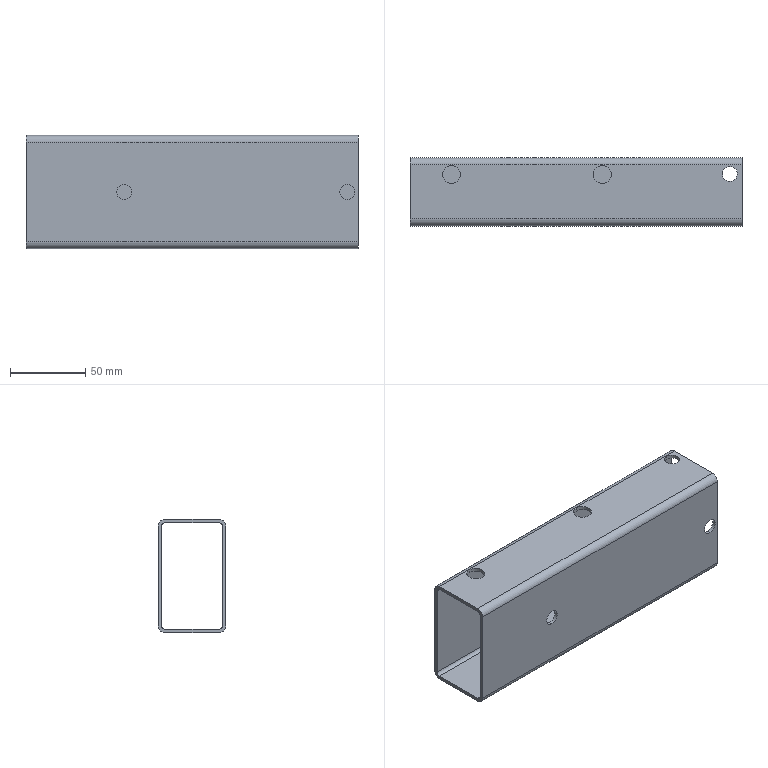Part | STEP file | [06] | 1 solid | 30 faces | box 220 x 45 x 75 mm | volume 112545 mm3 | cylinder 20 | plane 10 | commonest cylinder face diameters 10 x8 4.6 x4 9.2 x4 12 x4
STEP:
#1=CARTESIAN_POINT('',(65.,0.,42.5));
#2=VERTEX_POINT('',#1);
#3=CARTESIAN_POINT('',(65.,0.,32.5));
#4=VERTEX_POINT('',#3);
#5=CARTESIAN_POINT('',(65.,0.,37.5));
#6=DIRECTION('',(0.,1.,0.));
#7=DIRECTION('',(0.,0.,-1.));
#8=AXIS2_PLACEMENT_3D('',#5,#6,#7);
#9=CIRCLE('',#8,5.);
#10=EDGE_CURVE('',#2,#4,#9,.T.);
#11=ORIENTED_EDGE('',*,*,#10,.F.);
#12=CARTESIAN_POINT('',(65.,2.3,42.5));
#13=VERTEX_POINT('',#12);
#14=CARTESIAN_POINT('',(65.,0.,42.5));
#15=DIRECTION('',(0.,1.,0.));
#16=VECTOR('',#15,1000.);
#17=LINE('',#14,#16);
#18=EDGE_CURVE('',#2,#13,#17,.T.);
#19=ORIENTED_EDGE('',*,*,#18,.T.);
#20=CARTESIAN_POINT('',(65.,2.3,32.5));
#21=VERTEX_POINT('',#20);
#22=CARTESIAN_POINT('',(65.,2.3,37.5));
#23=DIRECTION('',(0.,-1.,0.));
#24=DIRECTION('',(0.,0.,1.));
#25=AXIS2_PLACEMENT_3D('',#22,#23,#24);
#26=CIRCLE('',#25,5.);
#27=EDGE_CURVE('',#21,#13,#26,.T.);
#28=ORIENTED_EDGE('',*,*,#27,.F.);
#29=CARTESIAN_POINT('',(65.,0.,32.5));
#30=DIRECTION('',(0.,1.,0.));
#31=VECTOR('',#30,1000.);
#32=LINE('',#29,#31);
#33=EDGE_CURVE('',#4,#21,#32,.T.);
#34=ORIENTED_EDGE('',*,*,#33,.F.);
#35=EDGE_LOOP('',(#11,#19,#28,#34));
#36=FACE_OUTER_BOUND('',#35,.T.);
#37=CARTESIAN_POINT('',(65.,0.,37.5));
#38=DIRECTION('',(0.,1.,0.));
#39=DIRECTION('',(0.,0.,-1.));
#40=AXIS2_PLACEMENT_3D('',#37,#38,#39);
#41=CYLINDRICAL_SURFACE('',#40,5.);
#42=ADVANCED_FACE('',(#36),#41,.F.);
#43=CARTESIAN_POINT('',(213.,0.,42.5));
#44=VERTEX_POINT('',#43);
#45=CARTESIAN_POINT('',(213.,0.,32.5));
#46=VERTEX_POINT('',#45);
#47=CARTESIAN_POINT('',(213.,0.,37.5));
#48=DIRECTION('',(0.,1.,0.));
#49=DIRECTION('',(0.,0.,-1.));
#50=AXIS2_PLACEMENT_3D('',#47,#48,#49);
#51=CIRCLE('',#50,5.);
#52=EDGE_CURVE('',#44,#46,#51,.T.);
#53=ORIENTED_EDGE('',*,*,#52,.F.);
#54=CARTESIAN_POINT('',(213.,2.3,42.5));
#55=VERTEX_POINT('',#54);
#56=CARTESIAN_POINT('',(213.,0.,42.5));
#57=DIRECTION('',(0.,1.,0.));
#58=VECTOR('',#57,1000.);
#59=LINE('',#56,#58);
#60=EDGE_CURVE('',#44,#55,#59,.T.);
#61=ORIENTED_EDGE('',*,*,#60,.T.);
#62=CARTESIAN_POINT('',(213.,2.3,32.5));
#63=VERTEX_POINT('',#62);
#64=CARTESIAN_POINT('',(213.,2.3,37.5));
#65=DIRECTION('',(0.,-1.,0.));
#66=DIRECTION('',(0.,0.,1.));
#67=AXIS2_PLACEMENT_3D('',#64,#65,#66);
#68=CIRCLE('',#67,5.);
#69=EDGE_CURVE('',#63,#55,#68,.T.);
#70=ORIENTED_EDGE('',*,*,#69,.F.);
#71=CARTESIAN_POINT('',(213.,0.,32.5));
#72=DIRECTION('',(0.,1.,0.));
#73=VECTOR('',#72,1000.);
#74=LINE('',#71,#73);
#75=EDGE_CURVE('',#46,#63,#74,.T.);
#76=ORIENTED_EDGE('',*,*,#75,.F.);
#77=EDGE_LOOP('',(#53,#61,#70,#76));
#78=FACE_OUTER_BOUND('',#77,.T.);
#79=CARTESIAN_POINT('',(213.,0.,37.5));
#80=DIRECTION('',(0.,1.,0.));
#81=DIRECTION('',(0.,0.,-1.));
#82=AXIS2_PLACEMENT_3D('',#79,#80,#81);
#83=CYLINDRICAL_SURFACE('',#82,5.);
#84=ADVANCED_FACE('',(#78),#83,.F.);
#85=CARTESIAN_POINT('',(212.,39.5,2.3));
#86=VERTEX_POINT('',#85);
#87=CARTESIAN_POINT('',(212.,29.5,2.3));
#88=VERTEX_POINT('',#87);
#89=CARTESIAN_POINT('',(212.,34.5,2.3));
#90=DIRECTION('',(0.,0.,-1.));
#91=DIRECTION('',(0.,-1.,0.));
#92=AXIS2_PLACEMENT_3D('',#89,#90,#91);
#93=CIRCLE('',#92,5.);
#94=EDGE_CURVE('',#86,#88,#93,.T.);
#95=ORIENTED_EDGE('',*,*,#94,.F.);
#96=CARTESIAN_POINT('',(212.,39.5,0.));
#97=VERTEX_POINT('',#96);
#98=CARTESIAN_POINT('',(212.,39.5,2.3));
#99=DIRECTION('',(0.,0.,-1.));
#100=VECTOR('',#99,1000.);
#101=LINE('',#98,#100);
#102=EDGE_CURVE('',#86,#97,#101,.T.);
#103=ORIENTED_EDGE('',*,*,#102,.T.);
#104=CARTESIAN_POINT('',(212.,29.5,0.));
#105=VERTEX_POINT('',#104);
#106=CARTESIAN_POINT('',(212.,34.5,0.));
#107=DIRECTION('',(0.,0.,1.));
#108=DIRECTION('',(0.,1.,0.));
#109=AXIS2_PLACEMENT_3D('',#106,#107,#108);
#110=CIRCLE('',#109,5.);
#111=EDGE_CURVE('',#105,#97,#110,.T.);
#112=ORIENTED_EDGE('',*,*,#111,.F.);
#113=CARTESIAN_POINT('',(212.,29.5,2.3));
#114=DIRECTION('',(0.,0.,-1.));
#115=VECTOR('',#114,1000.);
#116=LINE('',#113,#115);
#117=EDGE_CURVE('',#88,#105,#116,.T.);
#118=ORIENTED_EDGE('',*,*,#117,.F.);
#119=EDGE_LOOP('',(#95,#103,#112,#118));
#120=FACE_OUTER_BOUND('',#119,.T.);
#121=CARTESIAN_POINT('',(212.,34.5,2.3));
#122=DIRECTION('',(0.,0.,-1.));
#123=DIRECTION('',(0.,-1.,0.));
#124=AXIS2_PLACEMENT_3D('',#121,#122,#123);
#125=CYLINDRICAL_SURFACE('',#124,5.);
#126=ADVANCED_FACE('',(#120),#125,.F.);
#127=CARTESIAN_POINT('',(212.,39.5,75.));
#128=VERTEX_POINT('',#127);
#129=CARTESIAN_POINT('',(212.,29.5,75.));
#130=VERTEX_POINT('',#129);
#131=CARTESIAN_POINT('',(212.,34.5,75.));
#132=DIRECTION('',(0.,0.,-1.));
#133=DIRECTION('',(0.,-1.,0.));
#134=AXIS2_PLACEMENT_3D('',#131,#132,#133);
#135=CIRCLE('',#134,5.);
#136=EDGE_CURVE('',#128,#130,#135,.T.);
#137=ORIENTED_EDGE('',*,*,#136,.F.);
#138=CARTESIAN_POINT('',(212.,39.5,72.7));
#139=VERTEX_POINT('',#138);
#140=CARTESIAN_POINT('',(212.,39.5,75.));
#141=DIRECTION('',(0.,0.,-1.));
#142=VECTOR('',#141,1000.);
#143=LINE('',#140,#142);
#144=EDGE_CURVE('',#128,#139,#143,.T.);
#145=ORIENTED_EDGE('',*,*,#144,.T.);
#146=CARTESIAN_POINT('',(212.,29.5,72.7));
#147=VERTEX_POINT('',#146);
#148=CARTESIAN_POINT('',(212.,34.5,72.7));
#149=DIRECTION('',(0.,0.,1.));
#150=DIRECTION('',(0.,1.,0.));
#151=AXIS2_PLACEMENT_3D('',#148,#149,#150);
#152=CIRCLE('',#151,5.);
#153=EDGE_CURVE('',#147,#139,#152,.T.);
#154=ORIENTED_EDGE('',*,*,#153,.F.);
#155=CARTESIAN_POINT('',(212.,29.5,75.));
#156=DIRECTION('',(0.,0.,-1.));
#157=VECTOR('',#156,1000.);
#158=LINE('',#155,#157);
#159=EDGE_CURVE('',#130,#147,#158,.T.);
#160=ORIENTED_EDGE('',*,*,#159,.F.);
#161=EDGE_LOOP('',(#137,#145,#154,#160));
#162=FACE_OUTER_BOUND('',#161,.T.);
#163=CARTESIAN_POINT('',(212.,34.5,75.));
#164=DIRECTION('',(0.,0.,-1.));
#165=DIRECTION('',(0.,-1.,0.));
#166=AXIS2_PLACEMENT_3D('',#163,#164,#165);
#167=CYLINDRICAL_SURFACE('',#166,5.);
#168=ADVANCED_FACE('',(#162),#167,.F.);
#169=CARTESIAN_POINT('',(127.5,40.,75.));
#170=VERTEX_POINT('',#169);
#171=CARTESIAN_POINT('',(127.5,28.,75.));
#172=VERTEX_POINT('',#171);
#173=CARTESIAN_POINT('',(127.5,34.,75.));
#174=DIRECTION('',(0.,0.,-1.));
#175=DIRECTION('',(0.,-1.,0.));
#176=AXIS2_PLACEMENT_3D('',#173,#174,#175);
#177=CIRCLE('',#176,6.);
#178=EDGE_CURVE('',#170,#172,#177,.T.);
#179=ORIENTED_EDGE('',*,*,#178,.F.);
#180=CARTESIAN_POINT('',(127.5,40.,72.7));
#181=VERTEX_POINT('',#180);
#182=CARTESIAN_POINT('',(127.5,40.,75.));
#183=DIRECTION('',(0.,0.,-1.));
#184=VECTOR('',#183,1000.);
#185=LINE('',#182,#184);
#186=EDGE_CURVE('',#170,#181,#185,.T.);
#187=ORIENTED_EDGE('',*,*,#186,.T.);
#188=CARTESIAN_POINT('',(127.5,28.,72.7));
#189=VERTEX_POINT('',#188);
#190=CARTESIAN_POINT('',(127.5,34.,72.7));
#191=DIRECTION('',(0.,0.,1.));
#192=DIRECTION('',(0.,1.,0.));
#193=AXIS2_PLACEMENT_3D('',#190,#191,#192);
#194=CIRCLE('',#193,6.);
#195=EDGE_CURVE('',#189,#181,#194,.T.);
#196=ORIENTED_EDGE('',*,*,#195,.F.);
#197=CARTESIAN_POINT('',(127.5,28.,75.));
#198=DIRECTION('',(0.,0.,-1.));
#199=VECTOR('',#198,1000.);
#200=LINE('',#197,#199);
#201=EDGE_CURVE('',#172,#189,#200,.T.);
#202=ORIENTED_EDGE('',*,*,#201,.F.);
#203=EDGE_LOOP('',(#179,#187,#196,#202));
#204=FACE_OUTER_BOUND('',#203,.T.);
#205=CARTESIAN_POINT('',(127.5,34.,75.));
#206=DIRECTION('',(0.,0.,-1.));
#207=DIRECTION('',(0.,-1.,0.));
#208=AXIS2_PLACEMENT_3D('',#205,#206,#207);
#209=CYLINDRICAL_SURFACE('',#208,6.);
#210=ADVANCED_FACE('',(#204),#209,.F.);
#211=CARTESIAN_POINT('',(27.5,40.,75.));
#212=VERTEX_POINT('',#211);
#213=CARTESIAN_POINT('',(27.5,28.,75.));
#214=VERTEX_POINT('',#213);
#215=CARTESIAN_POINT('',(27.5,34.,75.));
#216=DIRECTION('',(0.,0.,-1.));
#217=DIRECTION('',(0.,-1.,0.));
#218=AXIS2_PLACEMENT_3D('',#215,#216,#217);
#219=CIRCLE('',#218,6.);
#220=EDGE_CURVE('',#212,#214,#219,.T.);
#221=ORIENTED_EDGE('',*,*,#220,.F.);
#222=CARTESIAN_POINT('',(27.5,40.,72.7));
#223=VERTEX_POINT('',#222);
#224=CARTESIAN_POINT('',(27.5,40.,75.));
#225=DIRECTION('',(0.,0.,-1.));
#226=VECTOR('',#225,1000.);
#227=LINE('',#224,#226);
#228=EDGE_CURVE('',#212,#223,#227,.T.);
#229=ORIENTED_EDGE('',*,*,#228,.T.);
#230=CARTESIAN_POINT('',(27.5,28.,72.7));
#231=VERTEX_POINT('',#230);
#232=CARTESIAN_POINT('',(27.5,34.,72.7));
#233=DIRECTION('',(0.,0.,1.));
#234=DIRECTION('',(0.,1.,0.));
#235=AXIS2_PLACEMENT_3D('',#232,#233,#234);
#236=CIRCLE('',#235,6.);
#237=EDGE_CURVE('',#231,#223,#236,.T.);
#238=ORIENTED_EDGE('',*,*,#237,.F.);
#239=CARTESIAN_POINT('',(27.5,28.,75.));
#240=DIRECTION('',(0.,0.,-1.));
#241=VECTOR('',#240,1000.);
#242=LINE('',#239,#241);
#243=EDGE_CURVE('',#214,#231,#242,.T.);
#244=ORIENTED_EDGE('',*,*,#243,.F.);
#245=EDGE_LOOP('',(#221,#229,#238,#244));
#246=FACE_OUTER_BOUND('',#245,.T.);
#247=CARTESIAN_POINT('',(27.5,34.,75.));
#248=DIRECTION('',(0.,0.,-1.));
#249=DIRECTION('',(0.,-1.,0.));
#250=AXIS2_PLACEMENT_3D('',#247,#248,#249);
#251=CYLINDRICAL_SURFACE('',#250,6.);
#252=ADVANCED_FACE('',(#246),#251,.F.);
#253=CARTESIAN_POINT('',(0.,45.,70.4));
#254=VERTEX_POINT('',#253);
#255=CARTESIAN_POINT('',(0.,45.,4.6));
#256=VERTEX_POINT('',#255);
#257=CARTESIAN_POINT('',(0.,45.,70.4));
#258=DIRECTION('',(0.,0.,-1.));
#259=VECTOR('',#258,1000.);
#260=LINE('',#257,#259);
#261=EDGE_CURVE('',#254,#256,#260,.T.);
#262=ORIENTED_EDGE('',*,*,#261,.T.);
#263=CARTESIAN_POINT('',(0.,40.4,0.));
#264=VERTEX_POINT('',#263);
#265=CARTESIAN_POINT('',(0.,40.4,4.6));
#266=DIRECTION('',(-1.,0.,0.));
#267=DIRECTION('',(0.,1.,0.));
#268=AXIS2_PLACEMENT_3D('',#265,#266,#267);
#269=CIRCLE('',#268,4.6);
#270=EDGE_CURVE('',#256,#264,#269,.T.);
#271=ORIENTED_EDGE('',*,*,#270,.T.);
#272=CARTESIAN_POINT('',(0.,4.6,0.));
#273=VERTEX_POINT('',#272);
#274=CARTESIAN_POINT('',(0.,40.4,0.));
#275=DIRECTION('',(0.,-1.,0.));
#276=VECTOR('',#275,1000.);
#277=LINE('',#274,#276);
#278=EDGE_CURVE('',#264,#273,#277,.T.);
#279=ORIENTED_EDGE('',*,*,#278,.T.);
#280=CARTESIAN_POINT('',(0.,0.,4.6));
#281=VERTEX_POINT('',#280);
#282=CARTESIAN_POINT('',(0.,4.6,4.6));
#283=DIRECTION('',(-1.,0.,0.));
#284=DIRECTION('',(0.,1.,0.));
#285=AXIS2_PLACEMENT_3D('',#282,#283,#284);
#286=CIRCLE('',#285,4.6);
#287=EDGE_CURVE('',#273,#281,#286,.T.);
#288=ORIENTED_EDGE('',*,*,#287,.T.);
#289=CARTESIAN_POINT('',(0.,0.,70.4));
#290=VERTEX_POINT('',#289);
#291=CARTESIAN_POINT('',(0.,0.,4.6));
#292=DIRECTION('',(0.,0.,1.));
#293=VECTOR('',#292,1000.);
#294=LINE('',#291,#293);
#295=EDGE_CURVE('',#281,#290,#294,.T.);
#296=ORIENTED_EDGE('',*,*,#295,.T.);
#297=CARTESIAN_POINT('',(0.,4.6,75.));
#298=VERTEX_POINT('',#297);
#299=CARTESIAN_POINT('',(0.,4.6,70.4));
#300=DIRECTION('',(-1.,0.,0.));
#301=DIRECTION('',(0.,1.,0.));
#302=AXIS2_PLACEMENT_3D('',#299,#300,#301);
#303=CIRCLE('',#302,4.6);
#304=EDGE_CURVE('',#290,#298,#303,.T.);
#305=ORIENTED_EDGE('',*,*,#304,.T.);
#306=CARTESIAN_POINT('',(0.,40.4,75.));
#307=VERTEX_POINT('',#306);
#308=CARTESIAN_POINT('',(0.,4.6,75.));
#309=DIRECTION('',(0.,1.,0.));
#310=VECTOR('',#309,1000.);
#311=LINE('',#308,#310);
#312=EDGE_CURVE('',#298,#307,#311,.T.);
#313=ORIENTED_EDGE('',*,*,#312,.T.);
#314=CARTESIAN_POINT('',(0.,40.4,70.4));
#315=DIRECTION('',(-1.,0.,0.));
#316=DIRECTION('',(0.,1.,0.));
#317=AXIS2_PLACEMENT_3D('',#314,#315,#316);
#318=CIRCLE('',#317,4.6);
#319=EDGE_CURVE('',#307,#254,#318,.T.);
#320=ORIENTED_EDGE('',*,*,#319,.T.);
#321=EDGE_LOOP('',(#262,#271,#279,#288,#296,#305,#313,#320));
#322=FACE_OUTER_BOUND('',#321,.T.);
#323=CARTESIAN_POINT('',(0.,42.7,70.4));
#324=VERTEX_POINT('',#323);
#325=CARTESIAN_POINT('',(0.,42.7,4.6));
#326=VERTEX_POINT('',#325);
#327=CARTESIAN_POINT('',(0.,42.7,70.4));
#328=DIRECTION('',(0.,0.,-1.));
#329=VECTOR('',#328,1000.);
#330=LINE('',#327,#329);
#331=EDGE_CURVE('',#324,#326,#330,.T.);
#332=ORIENTED_EDGE('',*,*,#331,.F.);
#333=CARTESIAN_POINT('',(0.,40.4,72.7));
#334=VERTEX_POINT('',#333);
#335=CARTESIAN_POINT('',(0.,40.4,70.4));
#336=DIRECTION('',(-1.,0.,0.));
#337=DIRECTION('',(0.,0.,1.));
#338=AXIS2_PLACEMENT_3D('',#335,#336,#337);
#339=CIRCLE('',#338,2.3);
#340=EDGE_CURVE('',#334,#324,#339,.T.);
#341=ORIENTED_EDGE('',*,*,#340,.F.);
#342=CARTESIAN_POINT('',(0.,4.6,72.7));
#343=VERTEX_POINT('',#342);
#344=CARTESIAN_POINT('',(0.,4.6,72.7));
#345=DIRECTION('',(0.,1.,0.));
#346=VECTOR('',#345,1000.);
#347=LINE('',#344,#346);
#348=EDGE_CURVE('',#343,#334,#347,.T.);
#349=ORIENTED_EDGE('',*,*,#348,.F.);
#350=CARTESIAN_POINT('',(0.,2.3,70.4));
#351=VERTEX_POINT('',#350);
#352=CARTESIAN_POINT('',(0.,4.6,70.4));
#353=DIRECTION('',(-1.,0.,0.));
#354=DIRECTION('',(0.,0.,1.));
#355=AXIS2_PLACEMENT_3D('',#352,#353,#354);
#356=CIRCLE('',#355,2.3);
#357=EDGE_CURVE('',#351,#343,#356,.T.);
#358=ORIENTED_EDGE('',*,*,#357,.F.);
#359=CARTESIAN_POINT('',(0.,2.3,4.6));
#360=VERTEX_POINT('',#359);
#361=CARTESIAN_POINT('',(0.,2.3,4.6));
#362=DIRECTION('',(0.,0.,1.));
#363=VECTOR('',#362,1000.);
#364=LINE('',#361,#363);
#365=EDGE_CURVE('',#360,#351,#364,.T.);
#366=ORIENTED_EDGE('',*,*,#365,.F.);
#367=CARTESIAN_POINT('',(0.,4.6,2.3));
#368=VERTEX_POINT('',#367);
#369=CARTESIAN_POINT('',(0.,4.6,4.6));
#370=DIRECTION('',(-1.,0.,0.));
#371=DIRECTION('',(0.,0.,1.));
#372=AXIS2_PLACEMENT_3D('',#369,#370,#371);
#373=CIRCLE('',#372,2.3);
#374=EDGE_CURVE('',#368,#360,#373,.T.);
#375=ORIENTED_EDGE('',*,*,#374,.F.);
#376=CARTESIAN_POINT('',(0.,40.4,2.3));
#377=VERTEX_POINT('',#376);
#378=CARTESIAN_POINT('',(0.,40.4,2.3));
#379=DIRECTION('',(0.,-1.,0.));
#380=VECTOR('',#379,1000.);
#381=LINE('',#378,#380);
#382=EDGE_CURVE('',#377,#368,#381,.T.);
#383=ORIENTED_EDGE('',*,*,#382,.F.);
#384=CARTESIAN_POINT('',(0.,40.4,4.6));
#385=DIRECTION('',(-1.,0.,0.));
#386=DIRECTION('',(0.,0.,1.));
#387=AXIS2_PLACEMENT_3D('',#384,#385,#386);
#388=CIRCLE('',#387,2.3);
#389=EDGE_CURVE('',#326,#377,#388,.T.);
#390=ORIENTED_EDGE('',*,*,#389,.F.);
#391=EDGE_LOOP('',(#332,#341,#349,#358,#366,#375,#383,#390));
#392=FACE_BOUND('',#391,.T.);
#393=CARTESIAN_POINT('',(0.,40.4,4.6));
#394=DIRECTION('',(-1.,0.,0.));
#395=DIRECTION('',(0.,1.,0.));
#396=AXIS2_PLACEMENT_3D('',#393,#394,#395);
#397=PLANE('',#396);
#398=ADVANCED_FACE('',(#322,#392),#397,.T.);
#399=CARTESIAN_POINT('',(220.,45.,70.4));
#400=VERTEX_POINT('',#399);
#401=CARTESIAN_POINT('',(220.,45.,4.6));
#402=VERTEX_POINT('',#401);
#403=CARTESIAN_POINT('',(220.,45.,70.4));
#404=DIRECTION('',(0.,0.,-1.));
#405=VECTOR('',#404,1000.);
#406=LINE('',#403,#405);
#407=EDGE_CURVE('',#400,#402,#406,.T.);
#408=ORIENTED_EDGE('',*,*,#407,.F.);
#409=CARTESIAN_POINT('',(220.,40.4,75.));
#410=VERTEX_POINT('',#409);
#411=CARTESIAN_POINT('',(220.,40.4,70.4));
#412=DIRECTION('',(-1.,0.,0.));
#413=DIRECTION('',(0.,1.,0.));
#414=AXIS2_PLACEMENT_3D('',#411,#412,#413);
#415=CIRCLE('',#414,4.6);
#416=EDGE_CURVE('',#410,#400,#415,.T.);
#417=ORIENTED_EDGE('',*,*,#416,.F.);
#418=CARTESIAN_POINT('',(220.,4.6,75.));
#419=VERTEX_POINT('',#418);
#420=CARTESIAN_POINT('',(220.,4.6,75.));
#421=DIRECTION('',(0.,1.,0.));
#422=VECTOR('',#421,1000.);
#423=LINE('',#420,#422);
#424=EDGE_CURVE('',#419,#410,#423,.T.);
#425=ORIENTED_EDGE('',*,*,#424,.F.);
#426=CARTESIAN_POINT('',(220.,0.,70.4));
#427=VERTEX_POINT('',#426);
#428=CARTESIAN_POINT('',(220.,4.6,70.4));
#429=DIRECTION('',(-1.,0.,0.));
#430=DIRECTION('',(0.,1.,0.));
#431=AXIS2_PLACEMENT_3D('',#428,#429,#430);
#432=CIRCLE('',#431,4.6);
#433=EDGE_CURVE('',#427,#419,#432,.T.);
#434=ORIENTED_EDGE('',*,*,#433,.F.);
#435=CARTESIAN_POINT('',(220.,0.,4.6));
#436=VERTEX_POINT('',#435);
#437=CARTESIAN_POINT('',(220.,0.,4.6));
#438=DIRECTION('',(0.,0.,1.));
#439=VECTOR('',#438,1000.);
#440=LINE('',#437,#439);
#441=EDGE_CURVE('',#436,#427,#440,.T.);
#442=ORIENTED_EDGE('',*,*,#441,.F.);
#443=CARTESIAN_POINT('',(220.,4.6,0.));
#444=VERTEX_POINT('',#443);
#445=CARTESIAN_POINT('',(220.,4.6,4.6));
#446=DIRECTION('',(-1.,0.,0.));
#447=DIRECTION('',(0.,1.,0.));
#448=AXIS2_PLACEMENT_3D('',#445,#446,#447);
#449=CIRCLE('',#448,4.6);
#450=EDGE_CURVE('',#444,#436,#449,.T.);
#451=ORIENTED_EDGE('',*,*,#450,.F.);
#452=CARTESIAN_POINT('',(220.,40.4,0.));
#453=VERTEX_POINT('',#452);
#454=CARTESIAN_POINT('',(220.,40.4,0.));
#455=DIRECTION('',(0.,-1.,0.));
#456=VECTOR('',#455,1000.);
#457=LINE('',#454,#456);
#458=EDGE_CURVE('',#453,#444,#457,.T.);
#459=ORIENTED_EDGE('',*,*,#458,.F.);
#460=CARTESIAN_POINT('',(220.,40.4,4.6));
#461=DIRECTION('',(-1.,0.,0.));
#462=DIRECTION('',(0.,1.,0.));
#463=AXIS2_PLACEMENT_3D('',#460,#461,#462);
#464=CIRCLE('',#463,4.6);
#465=EDGE_CURVE('',#402,#453,#464,.T.);
#466=ORIENTED_EDGE('',*,*,#465,.F.);
#467=EDGE_LOOP('',(#408,#417,#425,#434,#442,#451,#459,#466));
#468=FACE_OUTER_BOUND('',#467,.T.);
#469=CARTESIAN_POINT('',(220.,40.4,72.7));
#470=VERTEX_POINT('',#469);
#471=CARTESIAN_POINT('',(220.,42.7,70.4));
#472=VERTEX_POINT('',#471);
#473=CARTESIAN_POINT('',(220.,40.4,70.4));
#474=DIRECTION('',(-1.,0.,0.));
#475=DIRECTION('',(0.,0.,1.));
#476=AXIS2_PLACEMENT_3D('',#473,#474,#475);
#477=CIRCLE('',#476,2.3);
#478=EDGE_CURVE('',#470,#472,#477,.T.);
#479=ORIENTED_EDGE('',*,*,#478,.T.);
#480=CARTESIAN_POINT('',(220.,42.7,4.6));
#481=VERTEX_POINT('',#480);
#482=CARTESIAN_POINT('',(220.,42.7,70.4));
#483=DIRECTION('',(0.,0.,-1.));
#484=VECTOR('',#483,1000.);
#485=LINE('',#482,#484);
#486=EDGE_CURVE('',#472,#481,#485,.T.);
#487=ORIENTED_EDGE('',*,*,#486,.T.);
#488=CARTESIAN_POINT('',(220.,40.4,2.3));
#489=VERTEX_POINT('',#488);
#490=CARTESIAN_POINT('',(220.,40.4,4.6));
#491=DIRECTION('',(-1.,0.,0.));
#492=DIRECTION('',(0.,0.,1.));
#493=AXIS2_PLACEMENT_3D('',#490,#491,#492);
#494=CIRCLE('',#493,2.3);
#495=EDGE_CURVE('',#481,#489,#494,.T.);
#496=ORIENTED_EDGE('',*,*,#495,.T.);
#497=CARTESIAN_POINT('',(220.,4.6,2.3));
#498=VERTEX_POINT('',#497);
#499=CARTESIAN_POINT('',(220.,40.4,2.3));
#500=DIRECTION('',(0.,-1.,0.));
#501=VECTOR('',#500,1000.);
#502=LINE('',#499,#501);
#503=EDGE_CURVE('',#489,#498,#502,.T.);
#504=ORIENTED_EDGE('',*,*,#503,.T.);
#505=CARTESIAN_POINT('',(220.,2.3,4.6));
#506=VERTEX_POINT('',#505);
#507=CARTESIAN_POINT('',(220.,4.6,4.6));
#508=DIRECTION('',(-1.,0.,0.));
#509=DIRECTION('',(0.,0.,1.));
#510=AXIS2_PLACEMENT_3D('',#507,#508,#509);
#511=CIRCLE('',#510,2.3);
#512=EDGE_CURVE('',#498,#506,#511,.T.);
#513=ORIENTED_EDGE('',*,*,#512,.T.);
#514=CARTESIAN_POINT('',(220.,2.3,70.4));
#515=VERTEX_POINT('',#514);
#516=CARTESIAN_POINT('',(220.,2.3,4.6));
#517=DIRECTION('',(0.,0.,1.));
#518=VECTOR('',#517,1000.);
#519=LINE('',#516,#518);
#520=EDGE_CURVE('',#506,#515,#519,.T.);
#521=ORIENTED_EDGE('',*,*,#520,.T.);
#522=CARTESIAN_POINT('',(220.,4.6,72.7));
#523=VERTEX_POINT('',#522);
#524=CARTESIAN_POINT('',(220.,4.6,70.4));
#525=DIRECTION('',(-1.,0.,0.));
#526=DIRECTION('',(0.,0.,1.));
#527=AXIS2_PLACEMENT_3D('',#524,#525,#526);
#528=CIRCLE('',#527,2.3);
#529=EDGE_CURVE('',#515,#523,#528,.T.);
#530=ORIENTED_EDGE('',*,*,#529,.T.);
#531=CARTESIAN_POINT('',(220.,4.6,72.7));
#532=DIRECTION('',(0.,1.,0.));
#533=VECTOR('',#532,1000.);
#534=LINE('',#531,#533);
#535=EDGE_CURVE('',#523,#470,#534,.T.);
#536=ORIENTED_EDGE('',*,*,#535,.T.);
#537=EDGE_LOOP('',(#479,#487,#496,#504,#513,#521,#530,#536));
#538=FACE_BOUND('',#537,.T.);
#539=CARTESIAN_POINT('',(220.,40.4,4.6));
#540=DIRECTION('',(-1.,0.,0.));
#541=DIRECTION('',(0.,1.,0.));
#542=AXIS2_PLACEMENT_3D('',#539,#540,#541);
#543=PLANE('',#542);
#544=ADVANCED_FACE('',(#468,#538),#543,.F.);
#545=ORIENTED_EDGE('',*,*,#407,.T.);
#546=CARTESIAN_POINT('',(0.,45.,4.6));
#547=DIRECTION('',(1.,0.,0.));
#548=VECTOR('',#547,1000.);
#549=LINE('',#546,#548);
#550=EDGE_CURVE('',#256,#402,#549,.T.);
#551=ORIENTED_EDGE('',*,*,#550,.F.);
#552=ORIENTED_EDGE('',*,*,#261,.F.);
#553=CARTESIAN_POINT('',(0.,45.,70.4));
#554=DIRECTION('',(1.,0.,0.));
#555=VECTOR('',#554,1000.);
#556=LINE('',#553,#555);
#557=EDGE_CURVE('',#254,#400,#556,.T.);
#558=ORIENTED_EDGE('',*,*,#557,.T.);
#559=EDGE_LOOP('',(#545,#551,#552,#558));
#560=FACE_OUTER_BOUND('',#559,.T.);
#561=CARTESIAN_POINT('',(0.,45.,70.4));
#562=DIRECTION('',(0.,-1.,0.));
#563=DIRECTION('',(0.,0.,1.));
#564=AXIS2_PLACEMENT_3D('',#561,#562,#563);
#565=PLANE('',#564);
#566=ADVANCED_FACE('',(#560),#565,.F.);
#567=ORIENTED_EDGE('',*,*,#465,.T.);
#568=CARTESIAN_POINT('',(0.,40.4,0.));
#569=DIRECTION('',(1.,0.,0.));
#570=VECTOR('',#569,1000.);
#571=LINE('',#568,#570);
#572=EDGE_CURVE('',#264,#453,#571,.T.);
#573=ORIENTED_EDGE('',*,*,#572,.F.);
#574=ORIENTED_EDGE('',*,*,#270,.F.);
#575=ORIENTED_EDGE('',*,*,#550,.T.);
#576=EDGE_LOOP('',(#567,#573,#574,#575));
#577=FACE_OUTER_BOUND('',#576,.T.);
#578=CARTESIAN_POINT('',(0.,40.4,4.6));
#579=DIRECTION('',(1.,0.,0.));
#580=DIRECTION('',(0.,-1.,0.));
#581=AXIS2_PLACEMENT_3D('',#578,#579,#580);
#582=CYLINDRICAL_SURFACE('',#581,4.6);
#583=ADVANCED_FACE('',(#577),#582,.T.);
#584=ORIENTED_EDGE('',*,*,#111,.T.);
#585=CARTESIAN_POINT('',(212.,34.5,0.));
#586=DIRECTION('',(0.,0.,1.));
#587=DIRECTION('',(0.,1.,0.));
#588=AXIS2_PLACEMENT_3D('',#585,#586,#587);
#589=CIRCLE('',#588,5.);
#590=EDGE_CURVE('',#97,#105,#589,.T.);
#591=ORIENTED_EDGE('',*,*,#590,.T.);
#592=EDGE_LOOP('',(#584,#591));
#593=FACE_BOUND('',#592,.T.);
#594=ORIENTED_EDGE('',*,*,#458,.T.);
#595=CARTESIAN_POINT('',(0.,4.6,0.));
#596=DIRECTION('',(1.,0.,0.));
#597=VECTOR('',#596,1000.);
#598=LINE('',#595,#597);
#599=EDGE_CURVE('',#273,#444,#598,.T.);
#600=ORIENTED_EDGE('',*,*,#599,.F.);
#601=ORIENTED_EDGE('',*,*,#278,.F.);
#602=ORIENTED_EDGE('',*,*,#572,.T.);
#603=EDGE_LOOP('',(#594,#600,#601,#602));
#604=FACE_OUTER_BOUND('',#603,.T.);
#605=CARTESIAN_POINT('',(0.,40.4,0.));
#606=DIRECTION('',(0.,0.,1.));
#607=DIRECTION('',(0.,1.,0.));
#608=AXIS2_PLACEMENT_3D('',#605,#606,#607);
#609=PLANE('',#608);
#610=ADVANCED_FACE('',(#593,#604),#609,.F.);
#611=ORIENTED_EDGE('',*,*,#450,.T.);
#612=CARTESIAN_POINT('',(0.,0.,4.6));
#613=DIRECTION('',(1.,0.,0.));
#614=VECTOR('',#613,1000.);
#615=LINE('',#612,#614);
#616=EDGE_CURVE('',#281,#436,#615,.T.);
#617=ORIENTED_EDGE('',*,*,#616,.F.);
#618=ORIENTED_EDGE('',*,*,#287,.F.);
#619=ORIENTED_EDGE('',*,*,#599,.T.);
#620=EDGE_LOOP('',(#611,#617,#618,#619));
#621=FACE_OUTER_BOUND('',#620,.T.);
#622=CARTESIAN_POINT('',(0.,4.6,4.6));
#623=DIRECTION('',(1.,0.,0.));
#624=DIRECTION('',(0.,-1.,0.));
#625=AXIS2_PLACEMENT_3D('',#622,#623,#624);
#626=CYLINDRICAL_SURFACE('',#625,4.6);
#627=ADVANCED_FACE('',(#621),#626,.T.);
#628=CARTESIAN_POINT('',(65.,0.,37.5));
#629=DIRECTION('',(0.,1.,0.));
#630=DIRECTION('',(0.,0.,-1.));
#631=AXIS2_PLACEMENT_3D('',#628,#629,#630);
#632=CIRCLE('',#631,5.);
#633=EDGE_CURVE('',#4,#2,#632,.T.);
#634=ORIENTED_EDGE('',*,*,#633,.T.);
#635=ORIENTED_EDGE('',*,*,#10,.T.);
#636=EDGE_LOOP('',(#634,#635));
#637=FACE_BOUND('',#636,.T.);
#638=CARTESIAN_POINT('',(213.,0.,37.5));
#639=DIRECTION('',(0.,1.,0.));
#640=DIRECTION('',(0.,0.,-1.));
#641=AXIS2_PLACEMENT_3D('',#638,#639,#640);
#642=CIRCLE('',#641,5.);
#643=EDGE_CURVE('',#46,#44,#642,.T.);
#644=ORIENTED_EDGE('',*,*,#643,.T.);
#645=ORIENTED_EDGE('',*,*,#52,.T.);
#646=EDGE_LOOP('',(#644,#645));
#647=FACE_BOUND('',#646,.T.);
#648=ORIENTED_EDGE('',*,*,#441,.T.);
#649=CARTESIAN_POINT('',(0.,0.,70.4));
#650=DIRECTION('',(1.,0.,0.));
#651=VECTOR('',#650,1000.);
#652=LINE('',#649,#651);
#653=EDGE_CURVE('',#290,#427,#652,.T.);
#654=ORIENTED_EDGE('',*,*,#653,.F.);
#655=ORIENTED_EDGE('',*,*,#295,.F.);
#656=ORIENTED_EDGE('',*,*,#616,.T.);
#657=EDGE_LOOP('',(#648,#654,#655,#656));
#658=FACE_OUTER_BOUND('',#657,.T.);
#659=CARTESIAN_POINT('',(0.,0.,4.6));
#660=DIRECTION('',(0.,1.,0.));
#661=DIRECTION('',(0.,0.,-1.));
#662=AXIS2_PLACEMENT_3D('',#659,#660,#661);
#663=PLANE('',#662);
#664=ADVANCED_FACE('',(#637,#647,#658),#663,.F.);
#665=ORIENTED_EDGE('',*,*,#433,.T.);
#666=CARTESIAN_POINT('',(0.,4.6,75.));
#667=DIRECTION('',(1.,0.,0.));
#668=VECTOR('',#667,1000.);
#669=LINE('',#666,#668);
#670=EDGE_CURVE('',#298,#419,#669,.T.);
#671=ORIENTED_EDGE('',*,*,#670,.F.);
#672=ORIENTED_EDGE('',*,*,#304,.F.);
#673=ORIENTED_EDGE('',*,*,#653,.T.);
#674=EDGE_LOOP('',(#665,#671,#672,#673));
#675=FACE_OUTER_BOUND('',#674,.T.);
#676=CARTESIAN_POINT('',(0.,4.6,70.4));
#677=DIRECTION('',(1.,0.,0.));
#678=DIRECTION('',(0.,-1.,0.));
#679=AXIS2_PLACEMENT_3D('',#676,#677,#678);
#680=CYLINDRICAL_SURFACE('',#679,4.6);
#681=ADVANCED_FACE('',(#675),#680,.T.);
#682=CARTESIAN_POINT('',(212.,34.5,75.));
#683=DIRECTION('',(0.,0.,-1.));
#684=DIRECTION('',(0.,-1.,0.));
#685=AXIS2_PLACEMENT_3D('',#682,#683,#684);
#686=CIRCLE('',#685,5.);
#687=EDGE_CURVE('',#130,#128,#686,.T.);
#688=ORIENTED_EDGE('',*,*,#687,.T.);
#689=ORIENTED_EDGE('',*,*,#136,.T.);
#690=EDGE_LOOP('',(#688,#689));
#691=FACE_BOUND('',#690,.T.);
#692=CARTESIAN_POINT('',(127.5,34.,75.));
#693=DIRECTION('',(0.,0.,-1.));
#694=DIRECTION('',(0.,-1.,0.));
#695=AXIS2_PLACEMENT_3D('',#692,#693,#694);
#696=CIRCLE('',#695,6.);
#697=EDGE_CURVE('',#172,#170,#696,.T.);
#698=ORIENTED_EDGE('',*,*,#697,.T.);
#699=ORIENTED_EDGE('',*,*,#178,.T.);
#700=EDGE_LOOP('',(#698,#699));
#701=FACE_BOUND('',#700,.T.);
#702=CARTESIAN_POINT('',(27.5,34.,75.));
#703=DIRECTION('',(0.,0.,-1.));
#704=DIRECTION('',(0.,-1.,0.));
#705=AXIS2_PLACEMENT_3D('',#702,#703,#704);
#706=CIRCLE('',#705,6.);
#707=EDGE_CURVE('',#214,#212,#706,.T.);
#708=ORIENTED_EDGE('',*,*,#707,.T.);
#709=ORIENTED_EDGE('',*,*,#220,.T.);
#710=EDGE_LOOP('',(#708,#709));
#711=FACE_BOUND('',#710,.T.);
#712=ORIENTED_EDGE('',*,*,#424,.T.);
#713=CARTESIAN_POINT('',(0.,40.4,75.));
#714=DIRECTION('',(1.,0.,0.));
#715=VECTOR('',#714,1000.);
#716=LINE('',#713,#715);
#717=EDGE_CURVE('',#307,#410,#716,.T.);
#718=ORIENTED_EDGE('',*,*,#717,.F.);
#719=ORIENTED_EDGE('',*,*,#312,.F.);
#720=ORIENTED_EDGE('',*,*,#670,.T.);
#721=EDGE_LOOP('',(#712,#718,#719,#720));
#722=FACE_OUTER_BOUND('',#721,.T.);
#723=CARTESIAN_POINT('',(0.,4.6,75.));
#724=DIRECTION('',(0.,0.,-1.));
#725=DIRECTION('',(-1.,0.,0.));
#726=AXIS2_PLACEMENT_3D('',#723,#724,#725);
#727=PLANE('',#726);
#728=ADVANCED_FACE('',(#691,#701,#711,#722),#727,.F.);
#729=ORIENTED_EDGE('',*,*,#416,.T.);
#730=ORIENTED_EDGE('',*,*,#557,.F.);
#731=ORIENTED_EDGE('',*,*,#319,.F.);
#732=ORIENTED_EDGE('',*,*,#717,.T.);
#733=EDGE_LOOP('',(#729,#730,#731,#732));
#734=FACE_OUTER_BOUND('',#733,.T.);
#735=CARTESIAN_POINT('',(0.,40.4,70.4));
#736=DIRECTION('',(1.,0.,0.));
#737=DIRECTION('',(0.,-1.,0.));
#738=AXIS2_PLACEMENT_3D('',#735,#736,#737);
#739=CYLINDRICAL_SURFACE('',#738,4.6);
#740=ADVANCED_FACE('',(#734),#739,.T.);
#741=ORIENTED_EDGE('',*,*,#478,.F.);
#742=CARTESIAN_POINT('',(0.,40.4,72.7));
#743=DIRECTION('',(1.,0.,0.));
#744=VECTOR('',#743,1000.);
#745=LINE('',#742,#744);
#746=EDGE_CURVE('',#334,#470,#745,.T.);
#747=ORIENTED_EDGE('',*,*,#746,.F.);
#748=ORIENTED_EDGE('',*,*,#340,.T.);
#749=CARTESIAN_POINT('',(0.,42.7,70.4));
#750=DIRECTION('',(1.,0.,0.));
#751=VECTOR('',#750,1000.);
#752=LINE('',#749,#751);
#753=EDGE_CURVE('',#324,#472,#752,.T.);
#754=ORIENTED_EDGE('',*,*,#753,.T.);
#755=EDGE_LOOP('',(#741,#747,#748,#754));
#756=FACE_OUTER_BOUND('',#755,.T.);
#757=CARTESIAN_POINT('',(0.,40.4,70.4));
#758=DIRECTION('',(1.,0.,0.));
#759=DIRECTION('',(0.,0.,-1.));
#760=AXIS2_PLACEMENT_3D('',#757,#758,#759);
#761=CYLINDRICAL_SURFACE('',#760,2.3);
#762=ADVANCED_FACE('',(#756),#761,.F.);
#763=ORIENTED_EDGE('',*,*,#486,.F.);
#764=ORIENTED_EDGE('',*,*,#753,.F.);
#765=ORIENTED_EDGE('',*,*,#331,.T.);
#766=CARTESIAN_POINT('',(0.,42.7,4.6));
#767=DIRECTION('',(1.,0.,0.));
#768=VECTOR('',#767,1000.);
#769=LINE('',#766,#768);
#770=EDGE_CURVE('',#326,#481,#769,.T.);
#771=ORIENTED_EDGE('',*,*,#770,.T.);
#772=EDGE_LOOP('',(#763,#764,#765,#771));
#773=FACE_OUTER_BOUND('',#772,.T.);
#774=CARTESIAN_POINT('',(0.,42.7,70.4));
#775=DIRECTION('',(0.,-1.,0.));
#776=DIRECTION('',(1.,0.,0.));
#777=AXIS2_PLACEMENT_3D('',#774,#775,#776);
#778=PLANE('',#777);
#779=ADVANCED_FACE('',(#773),#778,.T.);
#780=ORIENTED_EDGE('',*,*,#495,.F.);
#781=ORIENTED_EDGE('',*,*,#770,.F.);
#782=ORIENTED_EDGE('',*,*,#389,.T.);
#783=CARTESIAN_POINT('',(0.,40.4,2.3));
#784=DIRECTION('',(1.,0.,0.));
#785=VECTOR('',#784,1000.);
#786=LINE('',#783,#785);
#787=EDGE_CURVE('',#377,#489,#786,.T.);
#788=ORIENTED_EDGE('',*,*,#787,.T.);
#789=EDGE_LOOP('',(#780,#781,#782,#788));
#790=FACE_OUTER_BOUND('',#789,.T.);
#791=CARTESIAN_POINT('',(0.,40.4,4.6));
#792=DIRECTION('',(1.,0.,0.));
#793=DIRECTION('',(0.,0.,-1.));
#794=AXIS2_PLACEMENT_3D('',#791,#792,#793);
#795=CYLINDRICAL_SURFACE('',#794,2.3);
#796=ADVANCED_FACE('',(#790),#795,.F.);
#797=CARTESIAN_POINT('',(212.,34.5,2.3));
#798=DIRECTION('',(0.,0.,-1.));
#799=DIRECTION('',(0.,-1.,0.));
#800=AXIS2_PLACEMENT_3D('',#797,#798,#799);
#801=CIRCLE('',#800,5.);
#802=EDGE_CURVE('',#88,#86,#801,.T.);
#803=ORIENTED_EDGE('',*,*,#802,.T.);
#804=ORIENTED_EDGE('',*,*,#94,.T.);
#805=EDGE_LOOP('',(#803,#804));
#806=FACE_BOUND('',#805,.T.);
#807=ORIENTED_EDGE('',*,*,#503,.F.);
#808=ORIENTED_EDGE('',*,*,#787,.F.);
#809=ORIENTED_EDGE('',*,*,#382,.T.);
#810=CARTESIAN_POINT('',(0.,4.6,2.3));
#811=DIRECTION('',(1.,0.,0.));
#812=VECTOR('',#811,1000.);
#813=LINE('',#810,#812);
#814=EDGE_CURVE('',#368,#498,#813,.T.);
#815=ORIENTED_EDGE('',*,*,#814,.T.);
#816=EDGE_LOOP('',(#807,#808,#809,#815));
#817=FACE_OUTER_BOUND('',#816,.T.);
#818=CARTESIAN_POINT('',(0.,40.4,2.3));
#819=DIRECTION('',(0.,0.,1.));
#820=DIRECTION('',(1.,0.,0.));
#821=AXIS2_PLACEMENT_3D('',#818,#819,#820);
#822=PLANE('',#821);
#823=ADVANCED_FACE('',(#806,#817),#822,.T.);
#824=ORIENTED_EDGE('',*,*,#512,.F.);
#825=ORIENTED_EDGE('',*,*,#814,.F.);
#826=ORIENTED_EDGE('',*,*,#374,.T.);
#827=CARTESIAN_POINT('',(0.,2.3,4.6));
#828=DIRECTION('',(1.,0.,0.));
#829=VECTOR('',#828,1000.);
#830=LINE('',#827,#829);
#831=EDGE_CURVE('',#360,#506,#830,.T.);
#832=ORIENTED_EDGE('',*,*,#831,.T.);
#833=EDGE_LOOP('',(#824,#825,#826,#832));
#834=FACE_OUTER_BOUND('',#833,.T.);
#835=CARTESIAN_POINT('',(0.,4.6,4.6));
#836=DIRECTION('',(1.,0.,0.));
#837=DIRECTION('',(0.,0.,-1.));
#838=AXIS2_PLACEMENT_3D('',#835,#836,#837);
#839=CYLINDRICAL_SURFACE('',#838,2.3);
#840=ADVANCED_FACE('',(#834),#839,.F.);
#841=ORIENTED_EDGE('',*,*,#27,.T.);
#842=CARTESIAN_POINT('',(65.,2.3,37.5));
#843=DIRECTION('',(0.,-1.,0.));
#844=DIRECTION('',(0.,0.,1.));
#845=AXIS2_PLACEMENT_3D('',#842,#843,#844);
#846=CIRCLE('',#845,5.);
#847=EDGE_CURVE('',#13,#21,#846,.T.);
#848=ORIENTED_EDGE('',*,*,#847,.T.);
#849=EDGE_LOOP('',(#841,#848));
#850=FACE_BOUND('',#849,.T.);
#851=ORIENTED_EDGE('',*,*,#69,.T.);
#852=CARTESIAN_POINT('',(213.,2.3,37.5));
#853=DIRECTION('',(0.,-1.,0.));
#854=DIRECTION('',(0.,0.,1.));
#855=AXIS2_PLACEMENT_3D('',#852,#853,#854);
#856=CIRCLE('',#855,5.);
#857=EDGE_CURVE('',#55,#63,#856,.T.);
#858=ORIENTED_EDGE('',*,*,#857,.T.);
#859=EDGE_LOOP('',(#851,#858));
#860=FACE_BOUND('',#859,.T.);
#861=ORIENTED_EDGE('',*,*,#520,.F.);
#862=ORIENTED_EDGE('',*,*,#831,.F.);
#863=ORIENTED_EDGE('',*,*,#365,.T.);
#864=CARTESIAN_POINT('',(0.,2.3,70.4));
#865=DIRECTION('',(1.,0.,0.));
#866=VECTOR('',#865,1000.);
#867=LINE('',#864,#866);
#868=EDGE_CURVE('',#351,#515,#867,.T.);
#869=ORIENTED_EDGE('',*,*,#868,.T.);
#870=EDGE_LOOP('',(#861,#862,#863,#869));
#871=FACE_OUTER_BOUND('',#870,.T.);
#872=CARTESIAN_POINT('',(0.,2.3,4.6));
#873=DIRECTION('',(0.,1.,0.));
#874=DIRECTION('',(0.,0.,-1.));
#875=AXIS2_PLACEMENT_3D('',#872,#873,#874);
#876=PLANE('',#875);
#877=ADVANCED_FACE('',(#850,#860,#871),#876,.T.);
#878=ORIENTED_EDGE('',*,*,#529,.F.);
#879=ORIENTED_EDGE('',*,*,#868,.F.);
#880=ORIENTED_EDGE('',*,*,#357,.T.);
#881=CARTESIAN_POINT('',(0.,4.6,72.7));
#882=DIRECTION('',(1.,0.,0.));
#883=VECTOR('',#882,1000.);
#884=LINE('',#881,#883);
#885=EDGE_CURVE('',#343,#523,#884,.T.);
#886=ORIENTED_EDGE('',*,*,#885,.T.);
#887=EDGE_LOOP('',(#878,#879,#880,#886));
#888=FACE_OUTER_BOUND('',#887,.T.);
#889=CARTESIAN_POINT('',(0.,4.6,70.4));
#890=DIRECTION('',(1.,0.,0.));
#891=DIRECTION('',(0.,0.,-1.));
#892=AXIS2_PLACEMENT_3D('',#889,#890,#891);
#893=CYLINDRICAL_SURFACE('',#892,2.3);
#894=ADVANCED_FACE('',(#888),#893,.F.);
#895=ORIENTED_EDGE('',*,*,#153,.T.);
#896=CARTESIAN_POINT('',(212.,34.5,72.7));
#897=DIRECTION('',(0.,0.,1.));
#898=DIRECTION('',(0.,1.,0.));
#899=AXIS2_PLACEMENT_3D('',#896,#897,#898);
#900=CIRCLE('',#899,5.);
#901=EDGE_CURVE('',#139,#147,#900,.T.);
#902=ORIENTED_EDGE('',*,*,#901,.T.);
#903=EDGE_LOOP('',(#895,#902));
#904=FACE_BOUND('',#903,.T.);
#905=ORIENTED_EDGE('',*,*,#195,.T.);
#906=CARTESIAN_POINT('',(127.5,34.,72.7));
#907=DIRECTION('',(0.,0.,1.));
#908=DIRECTION('',(0.,1.,0.));
#909=AXIS2_PLACEMENT_3D('',#906,#907,#908);
#910=CIRCLE('',#909,6.);
#911=EDGE_CURVE('',#181,#189,#910,.T.);
#912=ORIENTED_EDGE('',*,*,#911,.T.);
#913=EDGE_LOOP('',(#905,#912));
#914=FACE_BOUND('',#913,.T.);
#915=ORIENTED_EDGE('',*,*,#237,.T.);
#916=CARTESIAN_POINT('',(27.5,34.,72.7));
#917=DIRECTION('',(0.,0.,1.));
#918=DIRECTION('',(0.,1.,0.));
#919=AXIS2_PLACEMENT_3D('',#916,#917,#918);
#920=CIRCLE('',#919,6.);
#921=EDGE_CURVE('',#223,#231,#920,.T.);
#922=ORIENTED_EDGE('',*,*,#921,.T.);
#923=EDGE_LOOP('',(#915,#922));
#924=FACE_BOUND('',#923,.T.);
#925=ORIENTED_EDGE('',*,*,#535,.F.);
#926=ORIENTED_EDGE('',*,*,#885,.F.);
#927=ORIENTED_EDGE('',*,*,#348,.T.);
#928=ORIENTED_EDGE('',*,*,#746,.T.);
#929=EDGE_LOOP('',(#925,#926,#927,#928));
#930=FACE_OUTER_BOUND('',#929,.T.);
#931=CARTESIAN_POINT('',(0.,4.6,72.7));
#932=DIRECTION('',(0.,0.,-1.));
#933=DIRECTION('',(0.,-1.,0.));
#934=AXIS2_PLACEMENT_3D('',#931,#932,#933);
#935=PLANE('',#934);
#936=ADVANCED_FACE('',(#904,#914,#924,#930),#935,.T.);
#937=ORIENTED_EDGE('',*,*,#228,.F.);
#938=ORIENTED_EDGE('',*,*,#707,.F.);
#939=ORIENTED_EDGE('',*,*,#243,.T.);
#940=ORIENTED_EDGE('',*,*,#921,.F.);
#941=EDGE_LOOP('',(#937,#938,#939,#940));
#942=FACE_OUTER_BOUND('',#941,.T.);
#943=CARTESIAN_POINT('',(27.5,34.,75.));
#944=DIRECTION('',(0.,0.,-1.));
#945=DIRECTION('',(0.,-1.,0.));
#946=AXIS2_PLACEMENT_3D('',#943,#944,#945);
#947=CYLINDRICAL_SURFACE('',#946,6.);
#948=ADVANCED_FACE('',(#942),#947,.F.);
#949=ORIENTED_EDGE('',*,*,#186,.F.);
#950=ORIENTED_EDGE('',*,*,#697,.F.);
#951=ORIENTED_EDGE('',*,*,#201,.T.);
#952=ORIENTED_EDGE('',*,*,#911,.F.);
#953=EDGE_LOOP('',(#949,#950,#951,#952));
#954=FACE_OUTER_BOUND('',#953,.T.);
#955=CARTESIAN_POINT('',(127.5,34.,75.));
#956=DIRECTION('',(0.,0.,-1.));
#957=DIRECTION('',(0.,-1.,0.));
#958=AXIS2_PLACEMENT_3D('',#955,#956,#957);
#959=CYLINDRICAL_SURFACE('',#958,6.);
#960=ADVANCED_FACE('',(#954),#959,.F.);
#961=ORIENTED_EDGE('',*,*,#144,.F.);
#962=ORIENTED_EDGE('',*,*,#687,.F.);
#963=ORIENTED_EDGE('',*,*,#159,.T.);
#964=ORIENTED_EDGE('',*,*,#901,.F.);
#965=EDGE_LOOP('',(#961,#962,#963,#964));
#966=FACE_OUTER_BOUND('',#965,.T.);
#967=CARTESIAN_POINT('',(212.,34.5,75.));
#968=DIRECTION('',(0.,0.,-1.));
#969=DIRECTION('',(0.,-1.,0.));
#970=AXIS2_PLACEMENT_3D('',#967,#968,#969);
#971=CYLINDRICAL_SURFACE('',#970,5.);
#972=ADVANCED_FACE('',(#966),#971,.F.);
#973=ORIENTED_EDGE('',*,*,#102,.F.);
#974=ORIENTED_EDGE('',*,*,#802,.F.);
#975=ORIENTED_EDGE('',*,*,#117,.T.);
#976=ORIENTED_EDGE('',*,*,#590,.F.);
#977=EDGE_LOOP('',(#973,#974,#975,#976));
#978=FACE_OUTER_BOUND('',#977,.T.);
#979=CARTESIAN_POINT('',(212.,34.5,2.3));
#980=DIRECTION('',(0.,0.,-1.));
#981=DIRECTION('',(0.,-1.,0.));
#982=AXIS2_PLACEMENT_3D('',#979,#980,#981);
#983=CYLINDRICAL_SURFACE('',#982,5.);
#984=ADVANCED_FACE('',(#978),#983,.F.);
#985=ORIENTED_EDGE('',*,*,#60,.F.);
#986=ORIENTED_EDGE('',*,*,#643,.F.);
#987=ORIENTED_EDGE('',*,*,#75,.T.);
#988=ORIENTED_EDGE('',*,*,#857,.F.);
#989=EDGE_LOOP('',(#985,#986,#987,#988));
#990=FACE_OUTER_BOUND('',#989,.T.);
#991=CARTESIAN_POINT('',(213.,0.,37.5));
#992=DIRECTION('',(0.,1.,0.));
#993=DIRECTION('',(0.,0.,-1.));
#994=AXIS2_PLACEMENT_3D('',#991,#992,#993);
#995=CYLINDRICAL_SURFACE('',#994,5.);
#996=ADVANCED_FACE('',(#990),#995,.F.);
#997=ORIENTED_EDGE('',*,*,#18,.F.);
#998=ORIENTED_EDGE('',*,*,#633,.F.);
#999=ORIENTED_EDGE('',*,*,#33,.T.);
#1000=ORIENTED_EDGE('',*,*,#847,.F.);
#1001=EDGE_LOOP('',(#997,#998,#999,#1000));
#1002=FACE_OUTER_BOUND('',#1001,.T.);
#1003=CARTESIAN_POINT('',(65.,0.,37.5));
#1004=DIRECTION('',(0.,1.,0.));
#1005=DIRECTION('',(0.,0.,-1.));
#1006=AXIS2_PLACEMENT_3D('',#1003,#1004,#1005);
#1007=CYLINDRICAL_SURFACE('',#1006,5.);
#1008=ADVANCED_FACE('',(#1002),#1007,.F.);
#1009=CLOSED_SHELL('',(#42,#84,#126,#168,#210,#252,#398,#544,#566,#583,#610,#627,#664,#681,#728,#740,#762,#779,#796,#823,#840,#877,#894,#936,#948,#960,#972,#984,#996,#1008));
#1010=MANIFOLD_SOLID_BREP('',#1009);
#1011=CARTESIAN_POINT('',(0.,0.,0.));
#1012=DIRECTION('',(0.,0.,1.));
#1013=DIRECTION('',(1.,0.,0.));
#1014=AXIS2_PLACEMENT_3D('',#1011,#1012,#1013);
#1015=(LENGTH_UNIT()NAMED_UNIT(*)SI_UNIT(.MILLI.,.METRE.));
#1016=UNCERTAINTY_MEASURE_WITH_UNIT(LENGTH_MEASURE(0.00001),#1015,'','');
#1017=(NAMED_UNIT(*)PLANE_ANGLE_UNIT()SI_UNIT($,.RADIAN.));
#1018=(NAMED_UNIT(*)SI_UNIT($,.STERADIAN.)SOLID_ANGLE_UNIT());
#1019=(GEOMETRIC_REPRESENTATION_CONTEXT(3)GLOBAL_UNCERTAINTY_ASSIGNED_CONTEXT((#1016))GLOBAL_UNIT_ASSIGNED_CONTEXT((#1015,#1017,#1018))REPRESENTATION_CONTEXT('',''));
#1020=ADVANCED_BREP_SHAPE_REPRESENTATION('',(#1010,#1014),#1019);